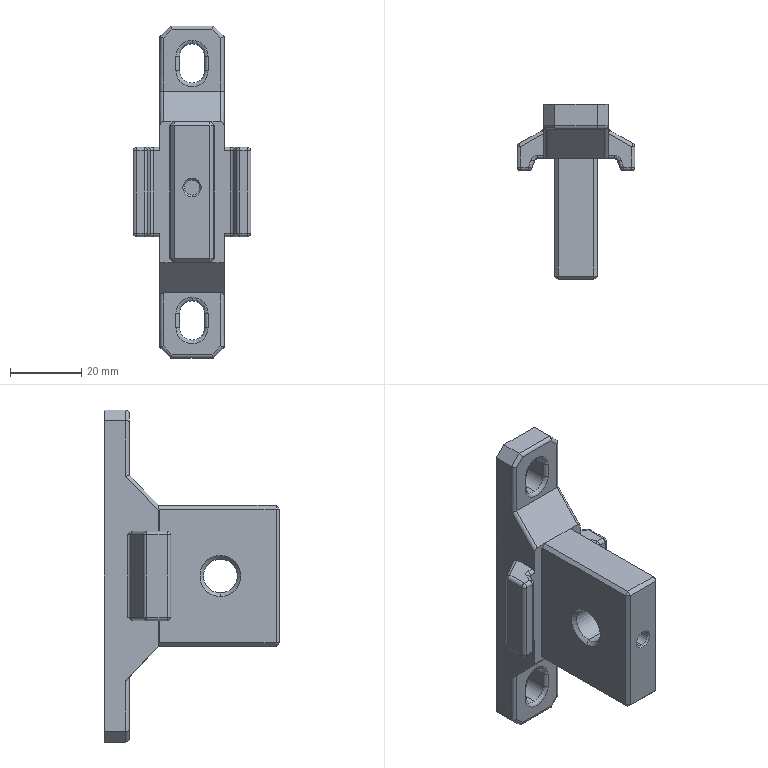Part | SolidWorks | features BaseBody 1 | 1 solid | 139 faces | box 33 x 49.1 x 93 mm | volume 35639 mm3 | cylinder 56 | plane 51 | spline 26 | cone 6 | commonest cylinder face diameters 2 x46 7 x6 4.2 x2 9.5 x2